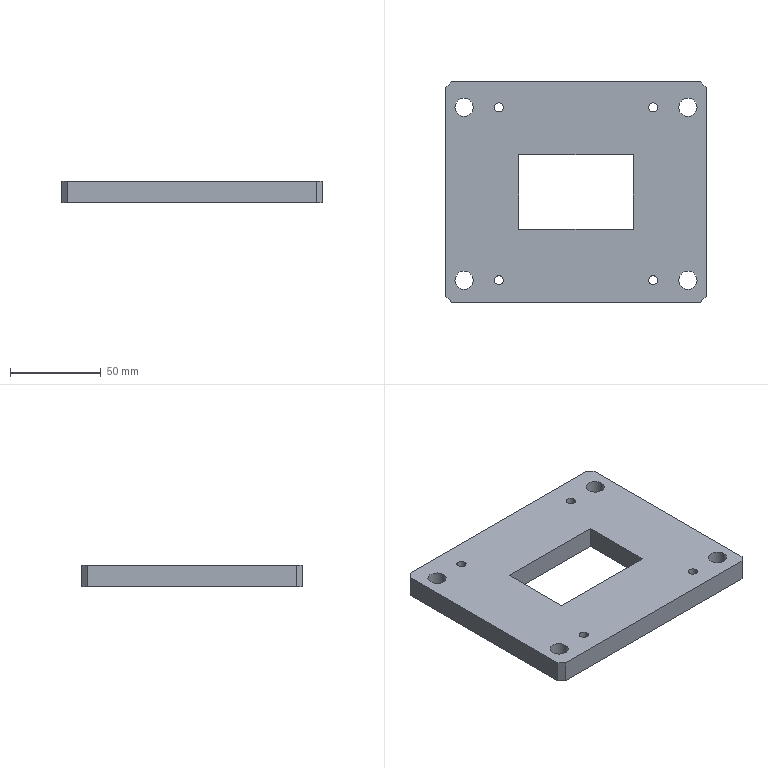Part | STEP file | 1 solid | 30 faces | box 143 x 121 x 12 mm | volume 171712 mm3 | cylinder 16 | plane 14 | commonest cylinder face diameters 5 x8 10 x8